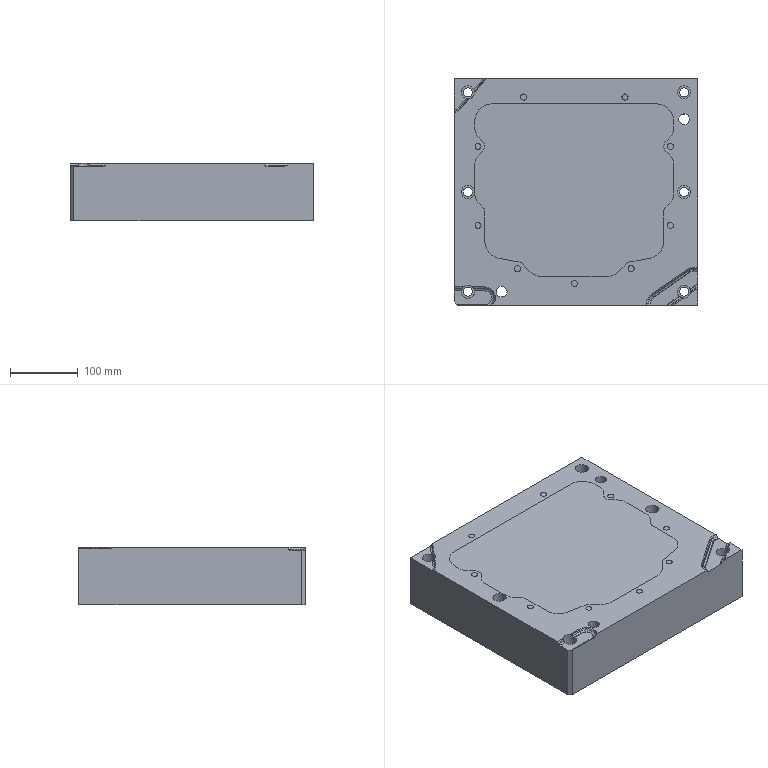Part | NX | features solid 2 | 1 solid | 80 faces | box 360.002 x 335.002 x 85 mm | volume 10067726 mm3 | plane 39 | cylinder 29 | spline 8 | cone 4 | commonest cylinder face diameters 6.2 x8 3.2 x7 13.5 x6 19.5 x6 16 x2